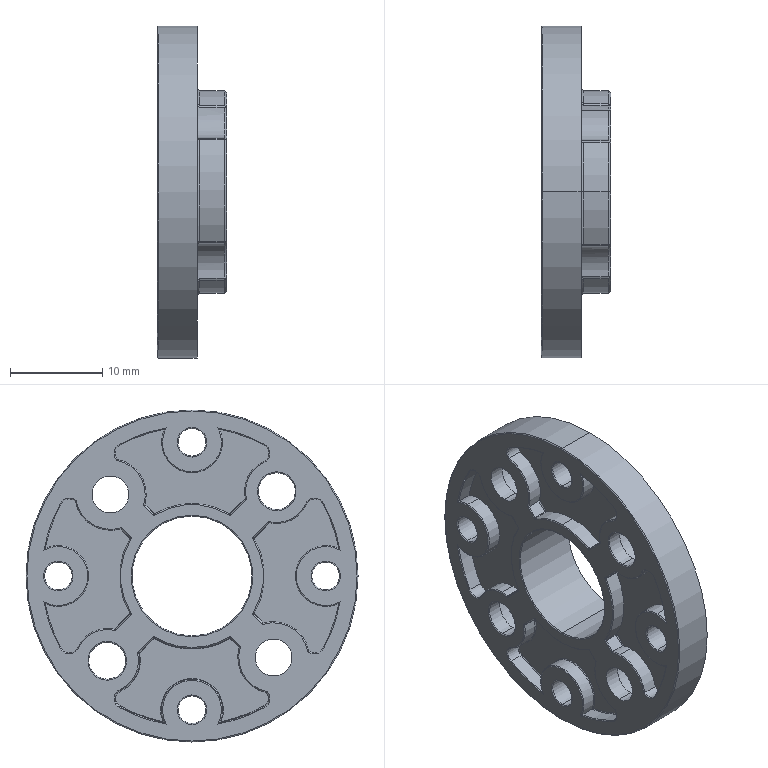Part | SolidWorks | features BaseBody 1 | 1 solid | 265 faces | box 7.5 x 36 x 36 mm | volume 3397 mm3 | cylinder 106 | torus 81 | plane 35 | cone 29 | spline 8 | sphere 6 | commonest cylinder face diameters 0.2 x31 2 x10 6.6 x9 3 x8 4 x8 6.7 x8